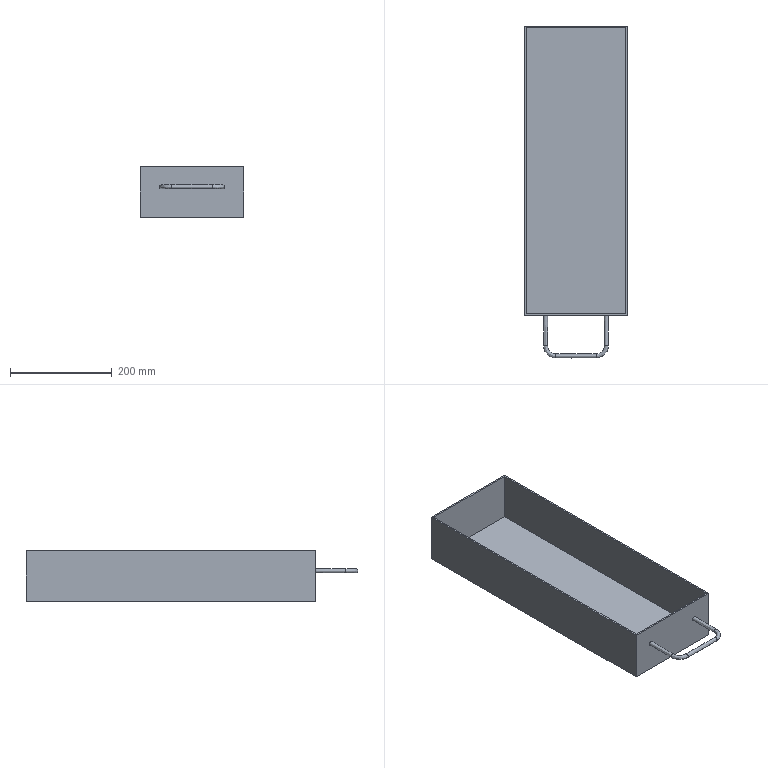Part | NX | features solid 2 | 1 solid | 16 faces | box 203 x 654 x 100 mm | volume 806741 mm3 | plane 11 | spline 5